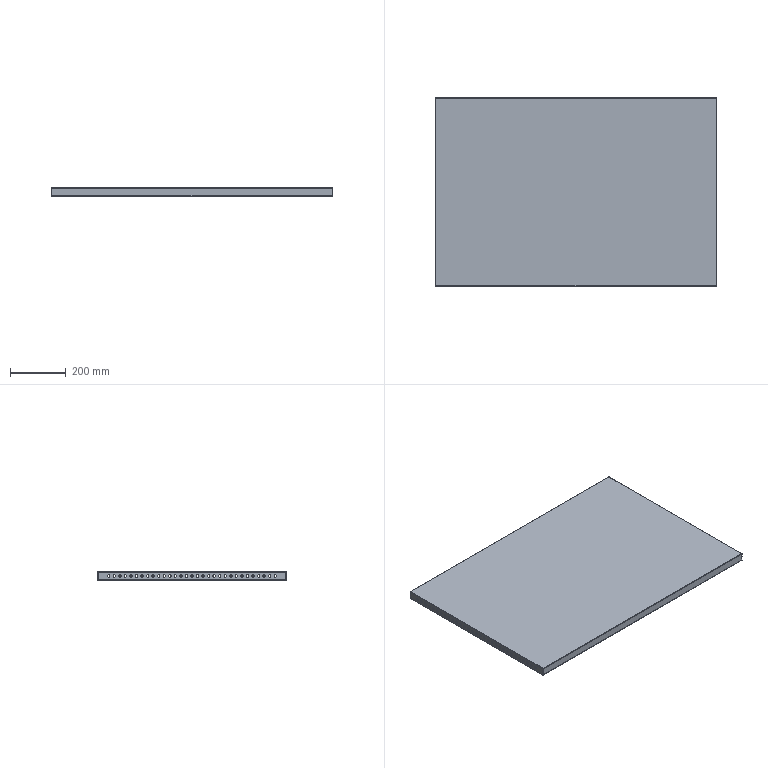Part | SolidWorks | features EdgeFlange 2, FlatPattern 1, ICE 1, SMBaseFlange 1, SheetMetal 1 | 1 solid | 194 faces | box 1016 x 680 x 30 mm | volume 1623193 mm3 | cylinder 140 | plane 38 | spline 16 | commonest cylinder face diameters 9 x124 0.2 x8 4.2 x8